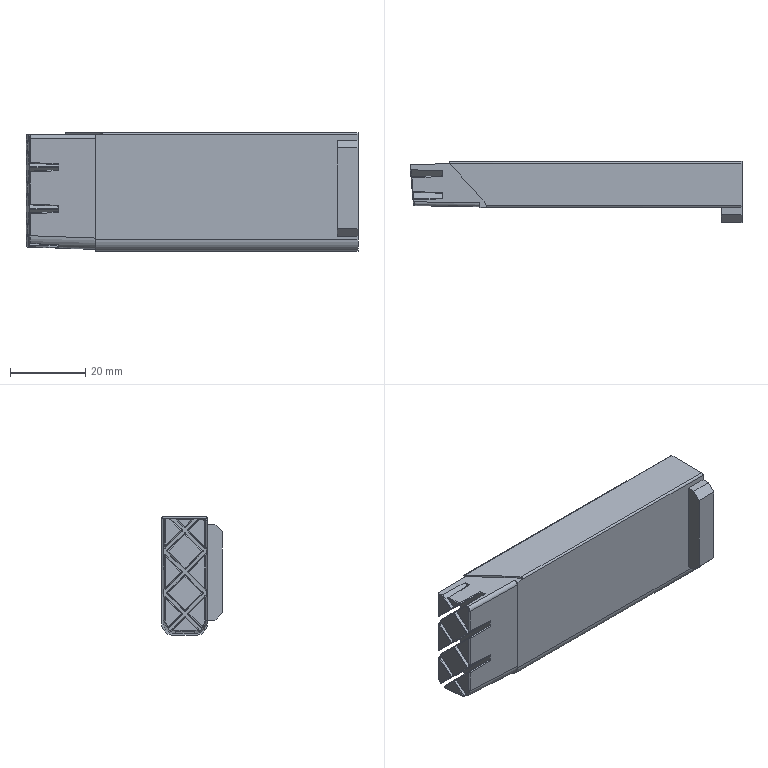Part | Creo | 1 solid | 213 faces | box 88.315 x 16.2 x 31.5 mm | volume 32583 mm3 | cylinder 70 | plane 63 | other 41 | sphere 31 | spline 8 | commonest cylinder face diameters 0.402 x61 1 x2 6 x2 6.03 x2 0.502 x1 2 x1